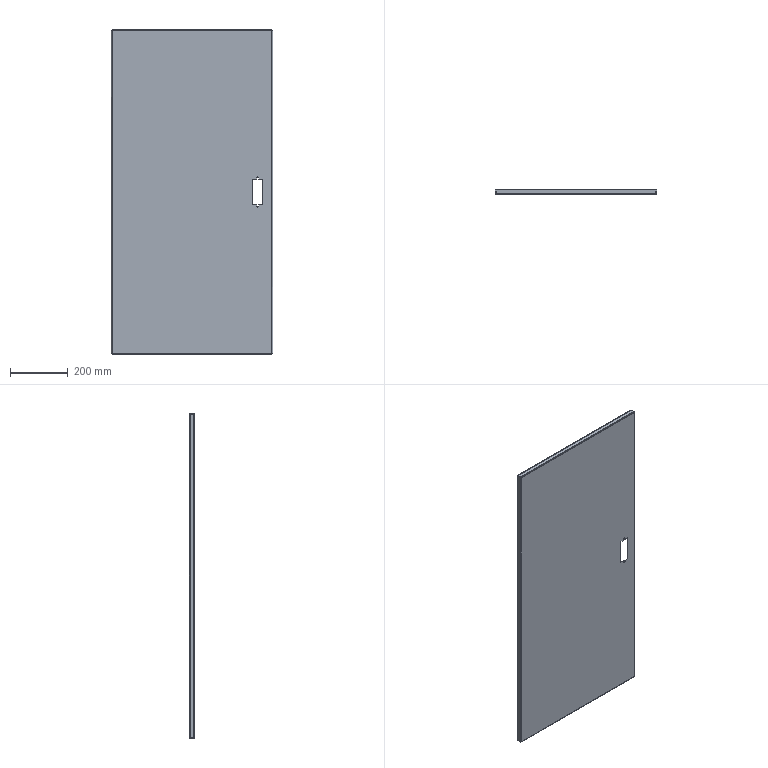Part | 1 solid | 83 faces | box 557 x 18 x 1121 mm | volume 1074529 mm3 | plane 48 | cylinder 19 | spline 16 | commonest cylinder face diameters 1.473 x8 4.473 x8 7 x3